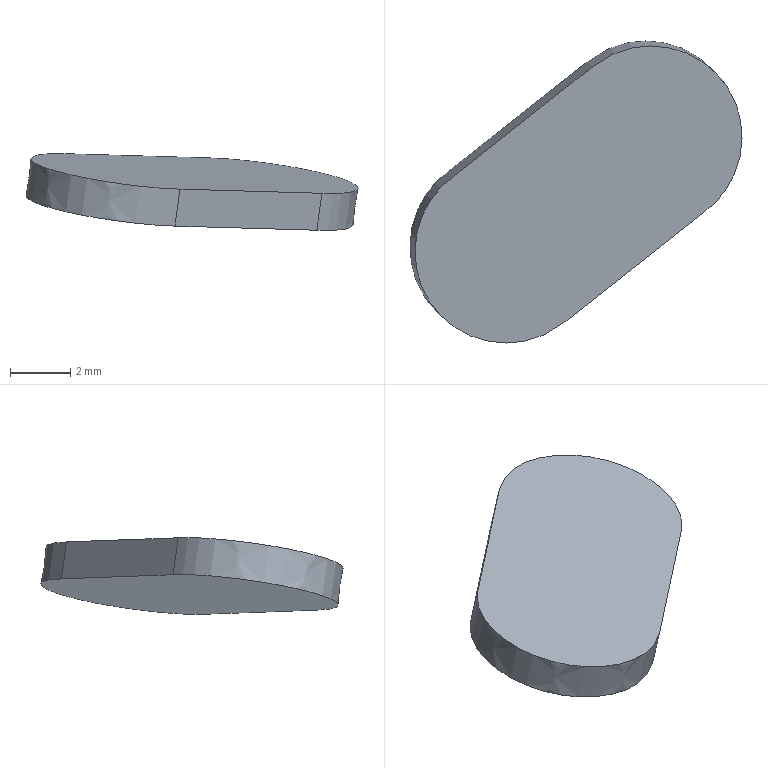Part | STEP file | gslz 2016.10.28-13_id1082_x_t | 1 solid | 6 faces | box 11.029 x 10.034 x 2.548 mm | volume 84.369 mm3 | other 2 | plane 2 | spline 2
STEP:
#1=CARTESIAN_POINT('',(0.,0.,0.));
#2=DIRECTION('',(0.,0.,1.));
#3=DIRECTION('',(1.,0.,0.));
#4=AXIS2_PLACEMENT_3D('',#1,#2,#3);
#5=CARTESIAN_POINT('',(753.441,156.947,-5.848));
#6=VERTEX_POINT('',#5);
#7=CARTESIAN_POINT('',(753.61,156.778,-4.621));
#8=VERTEX_POINT('',#7);
#9=CARTESIAN_POINT('',(753.441,156.947,-5.848));
#10=DIRECTION('',(0.1349,-0.1349,0.9816));
#11=VECTOR('',#10,1.);
#12=LINE('',#9,#11);
#13=CARTESIAN_POINT('',(753.441,156.947,-5.848));
#14=CARTESIAN_POINT('',(753.601,157.072,-5.852));
#15=CARTESIAN_POINT('',(753.942,157.297,-5.868));
#16=CARTESIAN_POINT('',(754.696,157.607,-5.929));
#17=CARTESIAN_POINT('',(755.723,157.678,-6.061));
#18=CARTESIAN_POINT('',(756.89,157.313,-6.271));
#19=CARTESIAN_POINT('',(757.817,156.519,-6.508));
#20=CARTESIAN_POINT('',(758.363,155.425,-6.733));
#21=CARTESIAN_POINT('',(758.438,154.2,-6.912));
#22=CARTESIAN_POINT('',(758.124,153.214,-7.004));
#23=CARTESIAN_POINT('',(757.644,152.553,-7.029));
#24=CARTESIAN_POINT('',(757.346,152.273,-7.027));
#25=CARTESIAN_POINT('',(757.187,152.148,-7.022));
#26=B_SPLINE_CURVE_WITH_KNOTS('',3,(#13,#14,#15,#16,#17,#18,#19,#20,#21,#22,#23,#24,#25),.UNSPECIFIED.,.F.,.F.,(4,1,1,1,1,1,1,1,1,1,4),(0.,0.0625,0.125,0.25,0.375,0.5,0.625,0.75,0.875,0.9375,1.),.UNSPECIFIED.);
#27=DIRECTION('',(0.1349,-0.1349,0.9816));
#28=VECTOR('',#27,1.);
#29=SURFACE_OF_LINEAR_EXTRUSION('',#26,#28);
#30=CARTESIAN_POINT('',(0.,0.));
#31=DIRECTION('',(0.,1.));
#32=VECTOR('',#31,1.);
#33=LINE('',#30,#32);
#34=(GEOMETRIC_REPRESENTATION_CONTEXT(2)PARAMETRIC_REPRESENTATION_CONTEXT()REPRESENTATION_CONTEXT('',''));
#35=DEFINITIONAL_REPRESENTATION('',(#33),#34);
#36=PCURVE('',#29,#35);
#37=CARTESIAN_POINT('',(748.729,153.235,-5.71));
#38=DIRECTION('',(0.6041,-0.7741,-0.1894));
#39=DIRECTION('',(0.7712,0.6278,-0.1058));
#40=AXIS2_PLACEMENT_3D('',#37,#38,#39);
#41=PLANE('',#40);
#42=CARTESIAN_POINT('',(5.979,0.5068));
#43=DIRECTION('',(-0.08446,0.9964));
#44=VECTOR('',#43,1.);
#45=LINE('',#42,#44);
#46=(GEOMETRIC_REPRESENTATION_CONTEXT(2)PARAMETRIC_REPRESENTATION_CONTEXT()REPRESENTATION_CONTEXT('',''));
#47=DEFINITIONAL_REPRESENTATION('',(#45),#46);
#48=PCURVE('',#41,#47);
#49=SURFACE_CURVE('',#12,(#36,#48),.PCURVE_S1.);
#50=EDGE_CURVE('',#6,#8,#49,.T.);
#51=ORIENTED_EDGE('',*,*,#50,.F.);
#52=CARTESIAN_POINT('',(757.187,152.148,-7.022));
#53=VERTEX_POINT('',#52);
#54=CARTESIAN_POINT('',(753.441,156.947,-5.848));
#55=CARTESIAN_POINT('',(753.711,157.16,-5.856));
#56=CARTESIAN_POINT('',(754.017,157.335,-5.873));
#57=CARTESIAN_POINT('',(754.339,157.452,-5.902));
#58=CARTESIAN_POINT('',(754.663,157.568,-5.93));
#59=CARTESIAN_POINT('',(755.012,157.625,-5.97));
#60=CARTESIAN_POINT('',(755.354,157.624,-6.017));
#61=CARTESIAN_POINT('',(755.681,157.623,-6.063));
#62=CARTESIAN_POINT('',(756.012,157.571,-6.115));
#63=CARTESIAN_POINT('',(756.321,157.47,-6.172));
#64=CARTESIAN_POINT('',(756.66,157.361,-6.233));
#65=CARTESIAN_POINT('',(756.982,157.188,-6.301));
#66=CARTESIAN_POINT('',(757.259,156.968,-6.37));
#67=CARTESIAN_POINT('',(757.524,156.757,-6.435));
#68=CARTESIAN_POINT('',(757.756,156.497,-6.503));
#69=CARTESIAN_POINT('',(757.935,156.209,-6.567));
#70=CARTESIAN_POINT('',(758.114,155.92,-6.631));
#71=CARTESIAN_POINT('',(758.247,155.595,-6.694));
#72=CARTESIAN_POINT('',(758.319,155.261,-6.75));
#73=CARTESIAN_POINT('',(758.391,154.929,-6.805));
#74=CARTESIAN_POINT('',(758.406,154.579,-6.855));
#75=CARTESIAN_POINT('',(758.367,154.24,-6.897));
#76=CARTESIAN_POINT('',(758.326,153.889,-6.939));
#77=CARTESIAN_POINT('',(758.227,153.539,-6.974));
#78=CARTESIAN_POINT('',(758.071,153.221,-6.996));
#79=CARTESIAN_POINT('',(757.917,152.909,-7.018));
#80=CARTESIAN_POINT('',(757.703,152.622,-7.028));
#81=CARTESIAN_POINT('',(757.453,152.38,-7.027));
#82=CARTESIAN_POINT('',(757.368,152.298,-7.026));
#83=CARTESIAN_POINT('',(757.279,152.221,-7.025));
#84=CARTESIAN_POINT('',(757.187,152.148,-7.022));
#85=B_SPLINE_CURVE_WITH_KNOTS('',3,(#54,#55,#56,#57,#58,#59,#60,#61,#62,#63,#64,#65,#66,#67,#68,#69,#70,#71,#72,#73,#74,#75,#76,#77,#78,#79,#80,#81,#82,#83,#84),.UNSPECIFIED.,.F.,.F.,(4,3,3,3,3,3,3,3,3,3,4),(0.,0.1062,0.213,0.315,0.4266,0.5332,0.6403,0.7466,0.8564,0.964,1.),.UNSPECIFIED.);
#86=CARTESIAN_POINT('',(0.,0.));
#87=DIRECTION('',(1.,0.));
#88=VECTOR('',#87,1.);
#89=LINE('',#86,#88);
#90=(GEOMETRIC_REPRESENTATION_CONTEXT(2)PARAMETRIC_REPRESENTATION_CONTEXT()REPRESENTATION_CONTEXT('',''));
#91=DEFINITIONAL_REPRESENTATION('',(#89),#90);
#92=PCURVE('',#29,#91);
#93=CARTESIAN_POINT('',(746.154,150.76,-5.696));
#94=CARTESIAN_POINT('',(747.778,149.136,-6.143));
#95=CARTESIAN_POINT('',(749.402,147.512,-6.589));
#96=CARTESIAN_POINT('',(751.026,145.888,-7.036));
#97=CARTESIAN_POINT('',(749.066,153.672,-5.696));
#98=CARTESIAN_POINT('',(750.69,152.048,-6.143));
#99=CARTESIAN_POINT('',(752.314,150.424,-6.589));
#100=CARTESIAN_POINT('',(753.938,148.8,-7.036));
#101=CARTESIAN_POINT('',(751.977,156.583,-5.696));
#102=CARTESIAN_POINT('',(753.601,154.959,-6.143));
#103=CARTESIAN_POINT('',(755.225,153.335,-6.589));
#104=CARTESIAN_POINT('',(756.849,151.711,-7.036));
#105=CARTESIAN_POINT('',(754.889,159.495,-5.696));
#106=CARTESIAN_POINT('',(756.513,157.871,-6.143));
#107=CARTESIAN_POINT('',(758.137,156.247,-6.589));
#108=CARTESIAN_POINT('',(759.761,154.623,-7.036));
#109=B_SPLINE_SURFACE_WITH_KNOTS('',3,3,((#93,#94,#95,#96),(#97,#98,#99,#100),(#101,#102,#103,#104),(#105,#106,#107,#108)),.UNSPECIFIED.,.F.,.F.,.F.,(4,4),(4,4),(0.,1.),(0.,1.),.PIECEWISE_BEZIER_KNOTS.);
#110=CARTESIAN_POINT('',(0.7713,0.1129));
#111=CARTESIAN_POINT('',(0.7772,0.1142));
#112=CARTESIAN_POINT('',(0.789,0.1174));
#113=CARTESIAN_POINT('',(0.8066,0.1243));
#114=CARTESIAN_POINT('',(0.8238,0.1332));
#115=CARTESIAN_POINT('',(0.8407,0.1443));
#116=CARTESIAN_POINT('',(0.8569,0.1575));
#117=CARTESIAN_POINT('',(0.8725,0.1729));
#118=CARTESIAN_POINT('',(0.8875,0.1905));
#119=CARTESIAN_POINT('',(0.9017,0.21));
#120=CARTESIAN_POINT('',(0.915,0.2312));
#121=CARTESIAN_POINT('',(0.9274,0.2539));
#122=CARTESIAN_POINT('',(0.9389,0.2782));
#123=CARTESIAN_POINT('',(0.9494,0.3039));
#124=CARTESIAN_POINT('',(0.959,0.3308));
#125=CARTESIAN_POINT('',(0.9674,0.3586));
#126=CARTESIAN_POINT('',(0.9747,0.3874));
#127=CARTESIAN_POINT('',(0.9808,0.4172));
#128=CARTESIAN_POINT('',(0.9856,0.4476));
#129=CARTESIAN_POINT('',(0.9893,0.4786));
#130=CARTESIAN_POINT('',(0.9916,0.5097));
#131=CARTESIAN_POINT('',(0.9927,0.5412));
#132=CARTESIAN_POINT('',(0.9924,0.5729));
#133=CARTESIAN_POINT('',(0.9909,0.6045));
#134=CARTESIAN_POINT('',(0.9881,0.6357));
#135=CARTESIAN_POINT('',(0.9841,0.6663));
#136=CARTESIAN_POINT('',(0.9788,0.6965));
#137=CARTESIAN_POINT('',(0.9723,0.7261));
#138=CARTESIAN_POINT('',(0.9646,0.7547));
#139=CARTESIAN_POINT('',(0.9558,0.7822));
#140=CARTESIAN_POINT('',(0.9458,0.8083));
#141=CARTESIAN_POINT('',(0.9348,0.8334));
#142=CARTESIAN_POINT('',(0.9228,0.857));
#143=CARTESIAN_POINT('',(0.9099,0.8791));
#144=CARTESIAN_POINT('',(0.8963,0.8995));
#145=CARTESIAN_POINT('',(0.8818,0.9182));
#146=CARTESIAN_POINT('',(0.8667,0.9352));
#147=CARTESIAN_POINT('',(0.8508,0.9502));
#148=CARTESIAN_POINT('',(0.8344,0.9632));
#149=CARTESIAN_POINT('',(0.8177,0.974));
#150=CARTESIAN_POINT('',(0.8004,0.9823));
#151=CARTESIAN_POINT('',(0.7827,0.9884));
#152=CARTESIAN_POINT('',(0.7648,0.9921));
#153=CARTESIAN_POINT('',(0.747,0.9937));
#154=CARTESIAN_POINT('',(0.729,0.993));
#155=CARTESIAN_POINT('',(0.7169,0.9911));
#156=CARTESIAN_POINT('',(0.7109,0.9898));
#157=B_SPLINE_CURVE_WITH_KNOTS('',3,(#110,#111,#112,#113,#114,#115,#116,#117,#118,#119,#120,#121,#122,#123,#124,#125,#126,#127,#128,#129,#130,#131,#132,#133,#134,#135,#136,#137,#138,#139,#140,#141,#142,#143,#144,#145,#146,#147,#148,#149,#150,#151,#152,#153,#154,#155,#156),.UNSPECIFIED.,.F.,.F.,(4,1,1,1,1,1,1,1,1,1,1,1,1,1,1,1,1,1,1,1,1,1,1,1,1,1,1,1,1,1,1,1,1,1,1,1,1,1,1,1,1,1,1,1,4),(0.,0.02273,0.04545,0.06818,0.09091,0.1136,0.1364,0.1591,0.1818,0.2045,0.2273,0.25,0.2727,0.2955,0.3182,0.3409,0.3636,0.3864,0.4091,0.4318,0.4545,0.4773,0.5,0.5227,0.5455,0.5682,0.5909,0.6136,0.6364,0.6591,0.6818,0.7045,0.7273,0.75,0.7727,0.7955,0.8182,0.8409,0.8636,0.8864,0.9091,0.9318,0.9545,0.9773,1.),.QUASI_UNIFORM_KNOTS.);
#158=(GEOMETRIC_REPRESENTATION_CONTEXT(2)PARAMETRIC_REPRESENTATION_CONTEXT()REPRESENTATION_CONTEXT('',''));
#159=DEFINITIONAL_REPRESENTATION('',(#157),#158);
#160=PCURVE('',#109,#159);
#161=SURFACE_CURVE('',#85,(#92,#160),.PCURVE_S1.);
#162=EDGE_CURVE('',#6,#53,#161,.T.);
#163=ORIENTED_EDGE('',*,*,#162,.T.);
#164=CARTESIAN_POINT('',(757.355,151.979,-5.795));
#165=VERTEX_POINT('',#164);
#166=CARTESIAN_POINT('',(757.187,152.148,-7.022));
#167=DIRECTION('',(0.1349,-0.1349,0.9816));
#168=VECTOR('',#167,1.);
#169=LINE('',#166,#168);
#170=CARTESIAN_POINT('',(1.,0.));
#171=DIRECTION('',(0.,1.));
#172=VECTOR('',#171,1.);
#173=LINE('',#170,#172);
#174=(GEOMETRIC_REPRESENTATION_CONTEXT(2)PARAMETRIC_REPRESENTATION_CONTEXT()REPRESENTATION_CONTEXT('',''));
#175=DEFINITIONAL_REPRESENTATION('',(#173),#174);
#176=PCURVE('',#29,#175);
#177=CARTESIAN_POINT('',(757.187,152.148,-7.022));
#178=DIRECTION('',(-0.6041,0.7741,0.1894));
#179=DIRECTION('',(-0.7712,-0.6278,0.1058));
#180=AXIS2_PLACEMENT_3D('',#177,#178,#179);
#181=PLANE('',#180);
#182=CARTESIAN_POINT('',(0.,0.));
#183=DIRECTION('',(0.08446,0.9964));
#184=VECTOR('',#183,1.);
#185=LINE('',#182,#184);
#186=(GEOMETRIC_REPRESENTATION_CONTEXT(2)PARAMETRIC_REPRESENTATION_CONTEXT()REPRESENTATION_CONTEXT('',''));
#187=DEFINITIONAL_REPRESENTATION('',(#185),#186);
#188=PCURVE('',#181,#187);
#189=SURFACE_CURVE('',#169,(#176,#188),.PCURVE_S1.);
#190=EDGE_CURVE('',#53,#165,#189,.T.);
#191=ORIENTED_EDGE('',*,*,#190,.T.);
#192=CARTESIAN_POINT('',(753.61,156.778,-4.621));
#193=CARTESIAN_POINT('',(753.88,156.991,-4.629));
#194=CARTESIAN_POINT('',(754.185,157.167,-4.646));
#195=CARTESIAN_POINT('',(754.508,157.283,-4.675));
#196=CARTESIAN_POINT('',(754.831,157.4,-4.703));
#197=CARTESIAN_POINT('',(755.18,157.457,-4.743));
#198=CARTESIAN_POINT('',(755.522,157.456,-4.79));
#199=CARTESIAN_POINT('',(755.85,157.455,-4.836));
#200=CARTESIAN_POINT('',(756.18,157.402,-4.888));
#201=CARTESIAN_POINT('',(756.49,157.302,-4.945));
#202=CARTESIAN_POINT('',(756.828,157.192,-5.006));
#203=CARTESIAN_POINT('',(757.151,157.02,-5.074));
#204=CARTESIAN_POINT('',(757.428,156.799,-5.143));
#205=CARTESIAN_POINT('',(757.693,156.588,-5.208));
#206=CARTESIAN_POINT('',(757.924,156.328,-5.275));
#207=CARTESIAN_POINT('',(758.103,156.04,-5.34));
#208=CARTESIAN_POINT('',(758.283,155.751,-5.404));
#209=CARTESIAN_POINT('',(758.416,155.426,-5.467));
#210=CARTESIAN_POINT('',(758.488,155.092,-5.523));
#211=CARTESIAN_POINT('',(758.559,154.76,-5.578));
#212=CARTESIAN_POINT('',(758.575,154.41,-5.628));
#213=CARTESIAN_POINT('',(758.535,154.071,-5.67));
#214=CARTESIAN_POINT('',(758.495,153.721,-5.712));
#215=CARTESIAN_POINT('',(758.396,153.37,-5.747));
#216=CARTESIAN_POINT('',(758.239,153.052,-5.769));
#217=CARTESIAN_POINT('',(758.086,152.741,-5.791));
#218=CARTESIAN_POINT('',(757.871,152.454,-5.801));
#219=CARTESIAN_POINT('',(757.622,152.212,-5.8));
#220=CARTESIAN_POINT('',(757.537,152.13,-5.799));
#221=CARTESIAN_POINT('',(757.448,152.052,-5.798));
#222=CARTESIAN_POINT('',(757.355,151.979,-5.795));
#223=B_SPLINE_CURVE_WITH_KNOTS('',3,(#192,#193,#194,#195,#196,#197,#198,#199,#200,#201,#202,#203,#204,#205,#206,#207,#208,#209,#210,#211,#212,#213,#214,#215,#216,#217,#218,#219,#220,#221,#222),.UNSPECIFIED.,.F.,.F.,(4,3,3,3,3,3,3,3,3,3,4),(0.,0.1062,0.213,0.315,0.4266,0.5332,0.6403,0.7466,0.8564,0.964,1.),.UNSPECIFIED.);
#224=CARTESIAN_POINT('',(0.,1.25));
#225=DIRECTION('',(1.,0.));
#226=VECTOR('',#225,1.);
#227=LINE('',#224,#226);
#228=(GEOMETRIC_REPRESENTATION_CONTEXT(2)PARAMETRIC_REPRESENTATION_CONTEXT()REPRESENTATION_CONTEXT('',''));
#229=DEFINITIONAL_REPRESENTATION('',(#227),#228);
#230=PCURVE('',#29,#229);
#231=CARTESIAN_POINT('',(582.842,140.622,16.631));
#232=CARTESIAN_POINT('',(603.987,119.477,10.818));
#233=CARTESIAN_POINT('',(625.133,98.331,5.005));
#234=CARTESIAN_POINT('',(646.279,77.185,-0.8076));
#235=CARTESIAN_POINT('',(667.424,56.039,-6.62));
#236=CARTESIAN_POINT('',(688.57,34.894,-12.433));
#237=CARTESIAN_POINT('',(618.357,176.138,16.631));
#238=CARTESIAN_POINT('',(639.503,154.992,10.818));
#239=CARTESIAN_POINT('',(660.649,133.847,5.005));
#240=CARTESIAN_POINT('',(681.795,112.701,-0.8078));
#241=CARTESIAN_POINT('',(702.94,91.555,-6.621));
#242=CARTESIAN_POINT('',(724.086,70.41,-12.434));
#243=CARTESIAN_POINT('',(653.873,211.654,16.631));
#244=CARTESIAN_POINT('',(675.019,190.508,10.818));
#245=CARTESIAN_POINT('',(696.165,169.363,5.005));
#246=CARTESIAN_POINT('',(717.31,148.217,-0.808));
#247=CARTESIAN_POINT('',(738.456,127.071,-6.621));
#248=CARTESIAN_POINT('',(759.602,105.925,-12.434));
#249=CARTESIAN_POINT('',(689.389,247.17,16.63));
#250=CARTESIAN_POINT('',(710.535,226.024,10.818));
#251=CARTESIAN_POINT('',(731.68,204.878,5.005));
#252=CARTESIAN_POINT('',(752.826,183.733,-0.8082));
#253=CARTESIAN_POINT('',(773.972,162.587,-6.621));
#254=CARTESIAN_POINT('',(795.118,141.441,-12.434));
#255=CARTESIAN_POINT('',(724.905,282.686,16.63));
#256=CARTESIAN_POINT('',(746.051,261.54,10.817));
#257=CARTESIAN_POINT('',(767.196,240.394,5.005));
#258=CARTESIAN_POINT('',(788.342,219.248,-0.8083));
#259=CARTESIAN_POINT('',(809.488,198.103,-6.621));
#260=CARTESIAN_POINT('',(830.633,176.957,-12.434));
#261=CARTESIAN_POINT('',(760.421,318.201,16.63));
#262=CARTESIAN_POINT('',(781.566,297.056,10.817));
#263=CARTESIAN_POINT('',(802.712,275.91,5.004));
#264=CARTESIAN_POINT('',(823.858,254.764,-0.8085));
#265=CARTESIAN_POINT('',(845.003,233.618,-6.621));
#266=CARTESIAN_POINT('',(866.149,212.473,-12.434));
#267=B_SPLINE_SURFACE_WITH_KNOTS('',5,5,((#231,#232,#233,#234,#235,#236),(#237,#238,#239,#240,#241,#242),(#243,#244,#245,#246,#247,#248),(#249,#250,#251,#252,#253,#254),(#255,#256,#257,#258,#259,#260),(#261,#262,#263,#264,#265,#266)),.UNSPECIFIED.,.F.,.F.,.F.,(6,6),(6,6),(0.,1.),(0.,1.),.PIECEWISE_BEZIER_KNOTS.);
#268=CARTESIAN_POINT('',(0.5263,0.7312));
#269=CARTESIAN_POINT('',(0.5266,0.7312));
#270=CARTESIAN_POINT('',(0.5272,0.7314));
#271=CARTESIAN_POINT('',(0.528,0.7317));
#272=CARTESIAN_POINT('',(0.5289,0.7321));
#273=CARTESIAN_POINT('',(0.5297,0.7326));
#274=CARTESIAN_POINT('',(0.5305,0.7332));
#275=CARTESIAN_POINT('',(0.5313,0.7339));
#276=CARTESIAN_POINT('',(0.532,0.7348));
#277=CARTESIAN_POINT('',(0.5327,0.7356));
#278=CARTESIAN_POINT('',(0.5334,0.7366));
#279=CARTESIAN_POINT('',(0.534,0.7377));
#280=CARTESIAN_POINT('',(0.5346,0.7388));
#281=CARTESIAN_POINT('',(0.5351,0.74));
#282=CARTESIAN_POINT('',(0.5355,0.7412));
#283=CARTESIAN_POINT('',(0.536,0.7425));
#284=CARTESIAN_POINT('',(0.5363,0.7438));
#285=CARTESIAN_POINT('',(0.5366,0.7452));
#286=CARTESIAN_POINT('',(0.5369,0.7466));
#287=CARTESIAN_POINT('',(0.537,0.748));
#288=CARTESIAN_POINT('',(0.5372,0.7495));
#289=CARTESIAN_POINT('',(0.5372,0.7509));
#290=CARTESIAN_POINT('',(0.5372,0.7524));
#291=CARTESIAN_POINT('',(0.5371,0.7538));
#292=CARTESIAN_POINT('',(0.537,0.7553));
#293=CARTESIAN_POINT('',(0.5368,0.7567));
#294=CARTESIAN_POINT('',(0.5365,0.7581));
#295=CARTESIAN_POINT('',(0.5362,0.7594));
#296=CARTESIAN_POINT('',(0.5358,0.7607));
#297=CARTESIAN_POINT('',(0.5354,0.762));
#298=CARTESIAN_POINT('',(0.5349,0.7632));
#299=CARTESIAN_POINT('',(0.5344,0.7644));
#300=CARTESIAN_POINT('',(0.5338,0.7655));
#301=CARTESIAN_POINT('',(0.5331,0.7665));
#302=CARTESIAN_POINT('',(0.5325,0.7674));
#303=CARTESIAN_POINT('',(0.5318,0.7683));
#304=CARTESIAN_POINT('',(0.531,0.7691));
#305=CARTESIAN_POINT('',(0.5302,0.7698));
#306=CARTESIAN_POINT('',(0.5294,0.7704));
#307=CARTESIAN_POINT('',(0.5286,0.7709));
#308=CARTESIAN_POINT('',(0.5277,0.7712));
#309=CARTESIAN_POINT('',(0.5269,0.7715));
#310=CARTESIAN_POINT('',(0.526,0.7717));
#311=CARTESIAN_POINT('',(0.5251,0.7718));
#312=CARTESIAN_POINT('',(0.5242,0.7717));
#313=CARTESIAN_POINT('',(0.5236,0.7716));
#314=CARTESIAN_POINT('',(0.5233,0.7716));
#315=B_SPLINE_CURVE_WITH_KNOTS('',3,(#268,#269,#270,#271,#272,#273,#274,#275,#276,#277,#278,#279,#280,#281,#282,#283,#284,#285,#286,#287,#288,#289,#290,#291,#292,#293,#294,#295,#296,#297,#298,#299,#300,#301,#302,#303,#304,#305,#306,#307,#308,#309,#310,#311,#312,#313,#314),.UNSPECIFIED.,.F.,.F.,(4,1,1,1,1,1,1,1,1,1,1,1,1,1,1,1,1,1,1,1,1,1,1,1,1,1,1,1,1,1,1,1,1,1,1,1,1,1,1,1,1,1,1,1,4),(0.,0.02273,0.04545,0.06818,0.09091,0.1136,0.1364,0.1591,0.1818,0.2045,0.2273,0.25,0.2727,0.2955,0.3182,0.3409,0.3636,0.3864,0.4091,0.4318,0.4545,0.4773,0.5,0.5227,0.5455,0.5682,0.5909,0.6136,0.6364,0.6591,0.6818,0.7045,0.7273,0.75,0.7727,0.7955,0.8182,0.8409,0.8636,0.8864,0.9091,0.9318,0.9545,0.9773,1.),.QUASI_UNIFORM_KNOTS.);
#316=(GEOMETRIC_REPRESENTATION_CONTEXT(2)PARAMETRIC_REPRESENTATION_CONTEXT()REPRESENTATION_CONTEXT('',''));
#317=DEFINITIONAL_REPRESENTATION('',(#315),#316);
#318=PCURVE('',#267,#317);
#319=SURFACE_CURVE('',#223,(#230,#318),.PCURVE_S1.);
#320=EDGE_CURVE('',#8,#165,#319,.T.);
#321=ORIENTED_EDGE('',*,*,#320,.F.);
#322=EDGE_LOOP('',(#51,#163,#191,#321));
#323=FACE_BOUND('',#322,.F.);
#324=ADVANCED_FACE('',(#323),#29,.F.);
#325=CARTESIAN_POINT('',(752.643,148.268,-5.657));
#326=VERTEX_POINT('',#325);
#327=CARTESIAN_POINT('',(757.355,151.979,-5.795));
#328=CARTESIAN_POINT('',(755.784,150.742,-5.749));
#329=CARTESIAN_POINT('',(754.214,149.505,-5.703));
#330=CARTESIAN_POINT('',(752.643,148.268,-5.657));
#331=B_SPLINE_CURVE_WITH_KNOTS('',3,(#327,#328,#329,#330),.UNSPECIFIED.,.F.,.F.,(4,4),(0.,1.),.PIECEWISE_BEZIER_KNOTS.);
#332=CARTESIAN_POINT('',(0.1056,1.246));
#333=CARTESIAN_POINT('',(2.098,1.077));
#334=CARTESIAN_POINT('',(4.091,0.9077));
#335=CARTESIAN_POINT('',(6.084,0.7388));
#336=B_SPLINE_CURVE_WITH_KNOTS('',3,(#332,#333,#334,#335),.UNSPECIFIED.,.F.,.F.,(4,4),(0.,1.),.PIECEWISE_BEZIER_KNOTS.);
#337=(GEOMETRIC_REPRESENTATION_CONTEXT(2)PARAMETRIC_REPRESENTATION_CONTEXT()REPRESENTATION_CONTEXT('',''));
#338=DEFINITIONAL_REPRESENTATION('',(#336),#337);
#339=PCURVE('',#181,#338);
#340=CARTESIAN_POINT('',(0.5233,0.7716));
#341=CARTESIAN_POINT('',(0.4996,0.7668));
#342=B_SPLINE_CURVE_WITH_KNOTS('',1,(#340,#341),.UNSPECIFIED.,.F.,.F.,(2,2),(0.,1.),.PIECEWISE_BEZIER_KNOTS.);
#343=(GEOMETRIC_REPRESENTATION_CONTEXT(2)PARAMETRIC_REPRESENTATION_CONTEXT()REPRESENTATION_CONTEXT('',''));
#344=DEFINITIONAL_REPRESENTATION('',(#342),#343);
#345=PCURVE('',#267,#344);
#346=SURFACE_CURVE('',#331,(#339,#345),.PCURVE_S1.);
#347=EDGE_CURVE('',#165,#326,#346,.T.);
#348=ORIENTED_EDGE('',*,*,#347,.T.);
#349=CARTESIAN_POINT('',(752.474,148.436,-6.884));
#350=VERTEX_POINT('',#349);
#351=CARTESIAN_POINT('',(752.474,148.436,-6.884));
#352=DIRECTION('',(0.1349,-0.1349,0.9816));
#353=VECTOR('',#352,1.);
#354=LINE('',#351,#353);
#355=CARTESIAN_POINT('',(5.979,-0.5068));
#356=DIRECTION('',(0.08446,0.9964));
#357=VECTOR('',#356,1.);
#358=LINE('',#355,#357);
#359=(GEOMETRIC_REPRESENTATION_CONTEXT(2)PARAMETRIC_REPRESENTATION_CONTEXT()REPRESENTATION_CONTEXT('',''));
#360=DEFINITIONAL_REPRESENTATION('',(#358),#359);
#361=PCURVE('',#181,#360);
#362=CARTESIAN_POINT('',(752.474,148.436,-6.884));
#363=CARTESIAN_POINT('',(752.315,148.311,-6.88));
#364=CARTESIAN_POINT('',(751.973,148.086,-6.864));
#365=CARTESIAN_POINT('',(751.22,147.776,-6.803));
#366=CARTESIAN_POINT('',(750.192,147.705,-6.671));
#367=CARTESIAN_POINT('',(749.026,148.07,-6.461));
#368=CARTESIAN_POINT('',(748.098,148.865,-6.224));
#369=CARTESIAN_POINT('',(747.552,149.959,-5.999));
#370=CARTESIAN_POINT('',(747.477,151.183,-5.82));
#371=CARTESIAN_POINT('',(747.792,152.169,-5.728));
#372=CARTESIAN_POINT('',(748.271,152.831,-5.703));
#373=CARTESIAN_POINT('',(748.569,153.11,-5.705));
#374=CARTESIAN_POINT('',(748.729,153.235,-5.71));
#375=B_SPLINE_CURVE_WITH_KNOTS('',3,(#362,#363,#364,#365,#366,#367,#368,#369,#370,#371,#372,#373,#374),.UNSPECIFIED.,.F.,.F.,(4,1,1,1,1,1,1,1,1,1,4),(0.,0.0625,0.125,0.25,0.375,0.5,0.625,0.75,0.875,0.9375,1.),.UNSPECIFIED.);
#376=DIRECTION('',(0.1349,-0.1349,0.9816));
#377=VECTOR('',#376,1.);
#378=SURFACE_OF_LINEAR_EXTRUSION('',#375,#377);
#379=CARTESIAN_POINT('',(0.,0.));
#380=DIRECTION('',(0.,1.));
#381=VECTOR('',#380,1.);
#382=LINE('',#379,#381);
#383=(GEOMETRIC_REPRESENTATION_CONTEXT(2)PARAMETRIC_REPRESENTATION_CONTEXT()REPRESENTATION_CONTEXT('',''));
#384=DEFINITIONAL_REPRESENTATION('',(#382),#383);
#385=PCURVE('',#378,#384);
#386=SURFACE_CURVE('',#354,(#361,#385),.PCURVE_S1.);
#387=EDGE_CURVE('',#350,#326,#386,.T.);
#388=ORIENTED_EDGE('',*,*,#387,.F.);
#389=CARTESIAN_POINT('',(757.187,152.148,-7.022));
#390=CARTESIAN_POINT('',(755.616,150.911,-6.976));
#391=CARTESIAN_POINT('',(754.045,149.673,-6.93));
#392=CARTESIAN_POINT('',(752.474,148.436,-6.884));
#393=B_SPLINE_CURVE_WITH_KNOTS('',3,(#389,#390,#391,#392),.UNSPECIFIED.,.F.,.F.,(4,4),(0.,1.),.PIECEWISE_BEZIER_KNOTS.);
#394=CARTESIAN_POINT('',(0.,0.));
#395=CARTESIAN_POINT('',(1.993,-0.1689));
#396=CARTESIAN_POINT('',(3.986,-0.3379));
#397=CARTESIAN_POINT('',(5.979,-0.5068));
#398=B_SPLINE_CURVE_WITH_KNOTS('',3,(#394,#395,#396,#397),.UNSPECIFIED.,.F.,.F.,(4,4),(0.,1.),.PIECEWISE_BEZIER_KNOTS.);
#399=(GEOMETRIC_REPRESENTATION_CONTEXT(2)PARAMETRIC_REPRESENTATION_CONTEXT()REPRESENTATION_CONTEXT('',''));
#400=DEFINITIONAL_REPRESENTATION('',(#398),#399);
#401=PCURVE('',#181,#400);
#402=CARTESIAN_POINT('',(0.7109,0.9898));
#403=CARTESIAN_POINT('',(0.2287,0.8871));
#404=B_SPLINE_CURVE_WITH_KNOTS('',1,(#402,#403),.UNSPECIFIED.,.F.,.F.,(2,2),(0.,1.),.PIECEWISE_BEZIER_KNOTS.);
#405=(GEOMETRIC_REPRESENTATION_CONTEXT(2)PARAMETRIC_REPRESENTATION_CONTEXT()REPRESENTATION_CONTEXT('',''));
#406=DEFINITIONAL_REPRESENTATION('',(#404),#405);
#407=PCURVE('',#109,#406);
#408=SURFACE_CURVE('',#393,(#401,#407),.PCURVE_S1.);
#409=EDGE_CURVE('',#53,#350,#408,.T.);
#410=ORIENTED_EDGE('',*,*,#409,.F.);
#411=ORIENTED_EDGE('',*,*,#190,.T.);
#412=EDGE_LOOP('',(#348,#388,#410,#411));
#413=FACE_BOUND('',#412,.T.);
#414=ADVANCED_FACE('',(#413),#181,.F.);
#415=ORIENTED_EDGE('',*,*,#387,.F.);
#416=CARTESIAN_POINT('',(748.729,153.235,-5.71));
#417=VERTEX_POINT('',#416);
#418=CARTESIAN_POINT('',(752.474,148.436,-6.884));
#419=CARTESIAN_POINT('',(752.204,148.224,-6.877));
#420=CARTESIAN_POINT('',(751.898,148.048,-6.859));
#421=CARTESIAN_POINT('',(751.576,147.932,-6.83));
#422=CARTESIAN_POINT('',(751.252,147.815,-6.802));
#423=CARTESIAN_POINT('',(750.903,147.758,-6.762));
#424=CARTESIAN_POINT('',(750.562,147.759,-6.715));
#425=CARTESIAN_POINT('',(750.234,147.76,-6.67));
#426=CARTESIAN_POINT('',(749.904,147.812,-6.617));
#427=CARTESIAN_POINT('',(749.594,147.913,-6.56));
#428=CARTESIAN_POINT('',(749.256,148.023,-6.499));
#429=CARTESIAN_POINT('',(748.933,148.195,-6.431));
#430=CARTESIAN_POINT('',(748.656,148.416,-6.363));
#431=CARTESIAN_POINT('',(748.391,148.627,-6.297));
#432=CARTESIAN_POINT('',(748.16,148.886,-6.23));
#433=CARTESIAN_POINT('',(747.981,149.174,-6.165));
#434=CARTESIAN_POINT('',(747.801,149.463,-6.101));
#435=CARTESIAN_POINT('',(747.668,149.788,-6.038));
#436=CARTESIAN_POINT('',(747.596,150.123,-5.982));
#437=CARTESIAN_POINT('',(747.525,150.455,-5.927));
#438=CARTESIAN_POINT('',(747.509,150.804,-5.877));
#439=CARTESIAN_POINT('',(747.548,151.144,-5.835));
#440=CARTESIAN_POINT('',(747.589,151.494,-5.793));
#441=CARTESIAN_POINT('',(747.688,151.844,-5.758));
#442=CARTESIAN_POINT('',(747.845,152.163,-5.736));
#443=CARTESIAN_POINT('',(747.998,152.474,-5.714));
#444=CARTESIAN_POINT('',(748.212,152.761,-5.704));
#445=CARTESIAN_POINT('',(748.462,153.003,-5.705));
#446=CARTESIAN_POINT('',(748.547,153.085,-5.706));
#447=CARTESIAN_POINT('',(748.636,153.163,-5.707));
#448=CARTESIAN_POINT('',(748.729,153.235,-5.71));
#449=B_SPLINE_CURVE_WITH_KNOTS('',3,(#418,#419,#420,#421,#422,#423,#424,#425,#426,#427,#428,#429,#430,#431,#432,#433,#434,#435,#436,#437,#438,#439,#440,#441,#442,#443,#444,#445,#446,#447,#448),.UNSPECIFIED.,.F.,.F.,(4,3,3,3,3,3,3,3,3,3,4),(0.,0.1062,0.213,0.315,0.4266,0.5332,0.6403,0.7466,0.8564,0.964,1.),.UNSPECIFIED.);
#450=CARTESIAN_POINT('',(0.,0.));
#451=DIRECTION('',(1.,0.));
#452=VECTOR('',#451,1.);
#453=LINE('',#450,#452);
#454=(GEOMETRIC_REPRESENTATION_CONTEXT(2)PARAMETRIC_REPRESENTATION_CONTEXT()REPRESENTATION_CONTEXT('',''));
#455=DEFINITIONAL_REPRESENTATION('',(#453),#454);
#456=PCURVE('',#378,#455);
#457=CARTESIAN_POINT('',(0.2287,0.8871));
#458=CARTESIAN_POINT('',(0.2228,0.8858));
#459=CARTESIAN_POINT('',(0.211,0.8826));
#460=CARTESIAN_POINT('',(0.1934,0.8757));
#461=CARTESIAN_POINT('',(0.1762,0.8668));
#462=CARTESIAN_POINT('',(0.1593,0.8557));
#463=CARTESIAN_POINT('',(0.1431,0.8425));
#464=CARTESIAN_POINT('',(0.1275,0.8271));
#465=CARTESIAN_POINT('',(0.1125,0.8095));
#466=CARTESIAN_POINT('',(0.09832,0.79));
#467=CARTESIAN_POINT('',(0.08501,0.7688));
#468=CARTESIAN_POINT('',(0.07264,0.7461));
#469=CARTESIAN_POINT('',(0.06112,0.7218));
#470=CARTESIAN_POINT('',(0.05055,0.6961));
#471=CARTESIAN_POINT('',(0.04102,0.6692));
#472=CARTESIAN_POINT('',(0.03259,0.6414));
#473=CARTESIAN_POINT('',(0.02535,0.6126));
#474=CARTESIAN_POINT('',(0.01924,0.5828));
#475=CARTESIAN_POINT('',(0.01435,0.5524));
#476=CARTESIAN_POINT('',(0.01071,0.5214));
#477=CARTESIAN_POINT('',(0.008384,0.4903));
#478=CARTESIAN_POINT('',(0.007344,0.4588));
#479=CARTESIAN_POINT('',(0.00758,0.4271));
#480=CARTESIAN_POINT('',(0.009087,0.3955));
#481=CARTESIAN_POINT('',(0.01186,0.3643));
#482=CARTESIAN_POINT('',(0.01589,0.3337));
#483=CARTESIAN_POINT('',(0.0212,0.3035));
#484=CARTESIAN_POINT('',(0.02772,0.2739));
#485=CARTESIAN_POINT('',(0.03541,0.2453));
#486=CARTESIAN_POINT('',(0.04423,0.2178));
#487=CARTESIAN_POINT('',(0.05416,0.1917));
#488=CARTESIAN_POINT('',(0.06519,0.1666));
#489=CARTESIAN_POINT('',(0.0772,0.143));
#490=CARTESIAN_POINT('',(0.09009,0.1209));
#491=CARTESIAN_POINT('',(0.1037,0.1005));
#492=CARTESIAN_POINT('',(0.1182,0.08181));
#493=CARTESIAN_POINT('',(0.1333,0.06483));
#494=CARTESIAN_POINT('',(0.1492,0.04976));
#495=CARTESIAN_POINT('',(0.1656,0.03676));
#496=CARTESIAN_POINT('',(0.1823,0.02602));
#497=CARTESIAN_POINT('',(0.1996,0.01766));
#498=CARTESIAN_POINT('',(0.2173,0.01161));
#499=CARTESIAN_POINT('',(0.2352,0.007852));
#500=CARTESIAN_POINT('',(0.253,0.006334));
#501=CARTESIAN_POINT('',(0.271,0.007038));
#502=CARTESIAN_POINT('',(0.2831,0.00891));
#503=CARTESIAN_POINT('',(0.2891,0.01018));
#504=B_SPLINE_CURVE_WITH_KNOTS('',3,(#457,#458,#459,#460,#461,#462,#463,#464,#465,#466,#467,#468,#469,#470,#471,#472,#473,#474,#475,#476,#477,#478,#479,#480,#481,#482,#483,#484,#485,#486,#487,#488,#489,#490,#491,#492,#493,#494,#495,#496,#497,#498,#499,#500,#501,#502,#503),.UNSPECIFIED.,.F.,.F.,(4,1,1,1,1,1,1,1,1,1,1,1,1,1,1,1,1,1,1,1,1,1,1,1,1,1,1,1,1,1,1,1,1,1,1,1,1,1,1,1,1,1,1,1,4),(0.,0.02273,0.04545,0.06818,0.09091,0.1136,0.1364,0.1591,0.1818,0.2045,0.2273,0.25,0.2727,0.2955,0.3182,0.3409,0.3636,0.3864,0.4091,0.4318,0.4545,0.4773,0.5,0.5227,0.5455,0.5682,0.5909,0.6136,0.6364,0.6591,0.6818,0.7045,0.7273,0.75,0.7727,0.7955,0.8182,0.8409,0.8636,0.8864,0.9091,0.9318,0.9545,0.9773,1.),.QUASI_UNIFORM_KNOTS.);
#505=(GEOMETRIC_REPRESENTATION_CONTEXT(2)PARAMETRIC_REPRESENTATION_CONTEXT()REPRESENTATION_CONTEXT('',''));
#506=DEFINITIONAL_REPRESENTATION('',(#504),#505);
#507=PCURVE('',#109,#506);
#508=SURFACE_CURVE('',#449,(#456,#507),.PCURVE_S1.);
#509=EDGE_CURVE('',#350,#417,#508,.T.);
#510=ORIENTED_EDGE('',*,*,#509,.T.);
#511=CARTESIAN_POINT('',(748.897,153.067,-4.483));
#512=VERTEX_POINT('',#511);
#513=CARTESIAN_POINT('',(748.729,153.235,-5.71));
#514=DIRECTION('',(0.1349,-0.1349,0.9816));
#515=VECTOR('',#514,1.);
#516=LINE('',#513,#515);
#517=CARTESIAN_POINT('',(1.,0.));
#518=DIRECTION('',(0.,1.));
#519=VECTOR('',#518,1.);
#520=LINE('',#517,#519);
#521=(GEOMETRIC_REPRESENTATION_CONTEXT(2)PARAMETRIC_REPRESENTATION_CONTEXT()REPRESENTATION_CONTEXT('',''));
#522=DEFINITIONAL_REPRESENTATION('',(#520),#521);
#523=PCURVE('',#378,#522);
#524=CARTESIAN_POINT('',(0.,0.));
#525=DIRECTION('',(-0.08446,0.9964));
#526=VECTOR('',#525,1.);
#527=LINE('',#524,#526);
#528=(GEOMETRIC_REPRESENTATION_CONTEXT(2)PARAMETRIC_REPRESENTATION_CONTEXT()REPRESENTATION_CONTEXT('',''));
#529=DEFINITIONAL_REPRESENTATION('',(#527),#528);
#530=PCURVE('',#41,#529);
#531=SURFACE_CURVE('',#516,(#523,#530),.PCURVE_S1.);
#532=EDGE_CURVE('',#417,#512,#531,.T.);
#533=ORIENTED_EDGE('',*,*,#532,.T.);
#534=CARTESIAN_POINT('',(752.643,148.268,-5.657));
#535=CARTESIAN_POINT('',(752.373,148.055,-5.65));
#536=CARTESIAN_POINT('',(752.067,147.879,-5.632));
#537=CARTESIAN_POINT('',(751.745,147.763,-5.603));
#538=CARTESIAN_POINT('',(751.421,147.646,-5.575));
#539=CARTESIAN_POINT('',(751.072,147.589,-5.535));
#540=CARTESIAN_POINT('',(750.73,147.59,-5.488));
#541=CARTESIAN_POINT('',(750.403,147.591,-5.443));
#542=CARTESIAN_POINT('',(750.072,147.644,-5.39));
#543=CARTESIAN_POINT('',(749.762,147.744,-5.333));
#544=CARTESIAN_POINT('',(749.424,147.854,-5.272));
#545=CARTESIAN_POINT('',(749.102,148.026,-5.204));
#546=CARTESIAN_POINT('',(748.825,148.247,-5.135));
#547=CARTESIAN_POINT('',(748.56,148.458,-5.07));
#548=CARTESIAN_POINT('',(748.328,148.718,-5.003));
#549=CARTESIAN_POINT('',(748.149,149.005,-4.938));
#550=CARTESIAN_POINT('',(747.969,149.295,-4.874));
#551=CARTESIAN_POINT('',(747.837,149.62,-4.811));
#552=CARTESIAN_POINT('',(747.765,149.954,-4.755));
#553=CARTESIAN_POINT('',(747.693,150.286,-4.7));
#554=CARTESIAN_POINT('',(747.678,150.635,-4.65));
#555=CARTESIAN_POINT('',(747.717,150.975,-4.608));
#556=CARTESIAN_POINT('',(747.757,151.325,-4.566));
#557=CARTESIAN_POINT('',(747.857,151.676,-4.531));
#558=CARTESIAN_POINT('',(748.013,151.994,-4.509));
#559=CARTESIAN_POINT('',(748.166,152.305,-4.487));
#560=CARTESIAN_POINT('',(748.381,152.592,-4.477));
#561=CARTESIAN_POINT('',(748.631,152.834,-4.478));
#562=CARTESIAN_POINT('',(748.716,152.916,-4.479));
#563=CARTESIAN_POINT('',(748.805,152.994,-4.48));
#564=CARTESIAN_POINT('',(748.897,153.067,-4.483));
#565=B_SPLINE_CURVE_WITH_KNOTS('',3,(#534,#535,#536,#537,#538,#539,#540,#541,#542,#543,#544,#545,#546,#547,#548,#549,#550,#551,#552,#553,#554,#555,#556,#557,#558,#559,#560,#561,#562,#563,#564),.UNSPECIFIED.,.F.,.F.,(4,3,3,3,3,3,3,3,3,3,4),(0.,0.1062,0.213,0.315,0.4266,0.5332,0.6403,0.7466,0.8564,0.964,1.),.UNSPECIFIED.);
#566=CARTESIAN_POINT('',(0.,1.25));
#567=DIRECTION('',(1.,0.));
#568=VECTOR('',#567,1.);
#569=LINE('',#566,#568);
#570=(GEOMETRIC_REPRESENTATION_CONTEXT(2)PARAMETRIC_REPRESENTATION_CONTEXT()REPRESENTATION_CONTEXT('',''));
#571=DEFINITIONAL_REPRESENTATION('',(#569),#570);
#572=PCURVE('',#378,#571);
#573=CARTESIAN_POINT('',(0.4996,0.7668));
#574=CARTESIAN_POINT('',(0.4993,0.7668));
#575=CARTESIAN_POINT('',(0.4988,0.7666));
#576=CARTESIAN_POINT('',(0.4979,0.7663));
#577=CARTESIAN_POINT('',(0.497,0.7659));
#578=CARTESIAN_POINT('',(0.4962,0.7654));
#579=CARTESIAN_POINT('',(0.4954,0.7648));
#580=CARTESIAN_POINT('',(0.4946,0.7641));
#581=CARTESIAN_POINT('',(0.4939,0.7633));
#582=CARTESIAN_POINT('',(0.4932,0.7624));
#583=CARTESIAN_POINT('',(0.4926,0.7614));
#584=CARTESIAN_POINT('',(0.4919,0.7604));
#585=CARTESIAN_POINT('',(0.4914,0.7592));
#586=CARTESIAN_POINT('',(0.4909,0.758));
#587=CARTESIAN_POINT('',(0.4904,0.7568));
#588=CARTESIAN_POINT('',(0.49,0.7555));
#589=CARTESIAN_POINT('',(0.4896,0.7542));
#590=CARTESIAN_POINT('',(0.4893,0.7528));
#591=CARTESIAN_POINT('',(0.4891,0.7514));
#592=CARTESIAN_POINT('',(0.4889,0.75));
#593=CARTESIAN_POINT('',(0.4888,0.7486));
#594=CARTESIAN_POINT('',(0.4887,0.7471));
#595=CARTESIAN_POINT('',(0.4887,0.7457));
#596=CARTESIAN_POINT('',(0.4888,0.7442));
#597=CARTESIAN_POINT('',(0.489,0.7428));
#598=CARTESIAN_POINT('',(0.4892,0.7413));
#599=CARTESIAN_POINT('',(0.4894,0.74));
#600=CARTESIAN_POINT('',(0.4897,0.7386));
#601=CARTESIAN_POINT('',(0.4901,0.7373));
#602=CARTESIAN_POINT('',(0.4906,0.736));
#603=CARTESIAN_POINT('',(0.491,0.7348));
#604=CARTESIAN_POINT('',(0.4916,0.7337));
#605=CARTESIAN_POINT('',(0.4922,0.7326));
#606=CARTESIAN_POINT('',(0.4928,0.7315));
#607=CARTESIAN_POINT('',(0.4935,0.7306));
#608=CARTESIAN_POINT('',(0.4942,0.7297));
#609=CARTESIAN_POINT('',(0.4949,0.729));
#610=CARTESIAN_POINT('',(0.4957,0.7283));
#611=CARTESIAN_POINT('',(0.4965,0.7277));
#612=CARTESIAN_POINT('',(0.4973,0.7272));
#613=CARTESIAN_POINT('',(0.4982,0.7268));
#614=CARTESIAN_POINT('',(0.4991,0.7265));
#615=CARTESIAN_POINT('',(0.4999,0.7263));
#616=CARTESIAN_POINT('',(0.5008,0.7263));
#617=CARTESIAN_POINT('',(0.5017,0.7263));
#618=CARTESIAN_POINT('',(0.5023,0.7264));
#619=CARTESIAN_POINT('',(0.5026,0.7264));
#620=B_SPLINE_CURVE_WITH_KNOTS('',3,(#573,#574,#575,#576,#577,#578,#579,#580,#581,#582,#583,#584,#585,#586,#587,#588,#589,#590,#591,#592,#593,#594,#595,#596,#597,#598,#599,#600,#601,#602,#603,#604,#605,#606,#607,#608,#609,#610,#611,#612,#613,#614,#615,#616,#617,#618,#619),.UNSPECIFIED.,.F.,.F.,(4,1,1,1,1,1,1,1,1,1,1,1,1,1,1,1,1,1,1,1,1,1,1,1,1,1,1,1,1,1,1,1,1,1,1,1,1,1,1,1,1,1,1,1,4),(0.,0.02273,0.04545,0.06818,0.09091,0.1136,0.1364,0.1591,0.1818,0.2045,0.2273,0.25,0.2727,0.2955,0.3182,0.3409,0.3636,0.3864,0.4091,0.4318,0.4545,0.4773,0.5,0.5227,0.5455,0.5682,0.5909,0.6136,0.6364,0.6591,0.6818,0.7045,0.7273,0.75,0.7727,0.7955,0.8182,0.8409,0.8636,0.8864,0.9091,0.9318,0.9545,0.9773,1.),.QUASI_UNIFORM_KNOTS.);
#621=(GEOMETRIC_REPRESENTATION_CONTEXT(2)PARAMETRIC_REPRESENTATION_CONTEXT()REPRESENTATION_CONTEXT('',''));
#622=DEFINITIONAL_REPRESENTATION('',(#620),#621);
#623=PCURVE('',#267,#622);
#624=SURFACE_CURVE('',#565,(#572,#623),.PCURVE_S1.);
#625=EDGE_CURVE('',#326,#512,#624,.T.);
#626=ORIENTED_EDGE('',*,*,#625,.F.);
#627=EDGE_LOOP('',(#415,#510,#533,#626));
#628=FACE_BOUND('',#627,.F.);
#629=ADVANCED_FACE('',(#628),#378,.F.);
#630=CARTESIAN_POINT('',(748.897,153.067,-4.483));
#631=CARTESIAN_POINT('',(750.468,154.304,-4.529));
#632=CARTESIAN_POINT('',(752.039,155.541,-4.575));
#633=CARTESIAN_POINT('',(753.61,156.778,-4.621));
#634=B_SPLINE_CURVE_WITH_KNOTS('',3,(#630,#631,#632,#633),.UNSPECIFIED.,.F.,.F.,(4,4),(0.,1.),.PIECEWISE_BEZIER_KNOTS.);
#635=CARTESIAN_POINT('',(-0.1056,1.246));
#636=CARTESIAN_POINT('',(1.887,1.414));
#637=CARTESIAN_POINT('',(3.88,1.583));
#638=CARTESIAN_POINT('',(5.873,1.752));
#639=B_SPLINE_CURVE_WITH_KNOTS('',3,(#635,#636,#637,#638),.UNSPECIFIED.,.F.,.F.,(4,4),(0.,1.),.PIECEWISE_BEZIER_KNOTS.);
#640=(GEOMETRIC_REPRESENTATION_CONTEXT(2)PARAMETRIC_REPRESENTATION_CONTEXT()REPRESENTATION_CONTEXT('',''));
#641=DEFINITIONAL_REPRESENTATION('',(#639),#640);
#642=PCURVE('',#41,#641);
#643=CARTESIAN_POINT('',(0.5026,0.7264));
#644=CARTESIAN_POINT('',(0.5263,0.7312));
#645=B_SPLINE_CURVE_WITH_KNOTS('',1,(#643,#644),.UNSPECIFIED.,.F.,.F.,(2,2),(0.,1.),.PIECEWISE_BEZIER_KNOTS.);
#646=(GEOMETRIC_REPRESENTATION_CONTEXT(2)PARAMETRIC_REPRESENTATION_CONTEXT()REPRESENTATION_CONTEXT('',''));
#647=DEFINITIONAL_REPRESENTATION('',(#645),#646);
#648=PCURVE('',#267,#647);
#649=SURFACE_CURVE('',#634,(#642,#648),.PCURVE_S1.);
#650=EDGE_CURVE('',#512,#8,#649,.T.);
#651=ORIENTED_EDGE('',*,*,#650,.T.);
#652=ORIENTED_EDGE('',*,*,#50,.F.);
#653=CARTESIAN_POINT('',(748.729,153.235,-5.71));
#654=CARTESIAN_POINT('',(750.299,154.473,-5.756));
#655=CARTESIAN_POINT('',(751.87,155.71,-5.802));
#656=CARTESIAN_POINT('',(753.441,156.947,-5.848));
#657=B_SPLINE_CURVE_WITH_KNOTS('',3,(#653,#654,#655,#656),.UNSPECIFIED.,.F.,.F.,(4,4),(0.,1.),.PIECEWISE_BEZIER_KNOTS.);
#658=CARTESIAN_POINT('',(0.,0.));
#659=CARTESIAN_POINT('',(1.993,0.1689));
#660=CARTESIAN_POINT('',(3.986,0.3379));
#661=CARTESIAN_POINT('',(5.979,0.5068));
#662=B_SPLINE_CURVE_WITH_KNOTS('',3,(#658,#659,#660,#661),.UNSPECIFIED.,.F.,.F.,(4,4),(0.,1.),.PIECEWISE_BEZIER_KNOTS.);
#663=(GEOMETRIC_REPRESENTATION_CONTEXT(2)PARAMETRIC_REPRESENTATION_CONTEXT()REPRESENTATION_CONTEXT('',''));
#664=DEFINITIONAL_REPRESENTATION('',(#662),#663);
#665=PCURVE('',#41,#664);
#666=CARTESIAN_POINT('',(0.2891,0.01018));
#667=CARTESIAN_POINT('',(0.7713,0.1129));
#668=B_SPLINE_CURVE_WITH_KNOTS('',1,(#666,#667),.UNSPECIFIED.,.F.,.F.,(2,2),(0.,1.),.PIECEWISE_BEZIER_KNOTS.);
#669=(GEOMETRIC_REPRESENTATION_CONTEXT(2)PARAMETRIC_REPRESENTATION_CONTEXT()REPRESENTATION_CONTEXT('',''));
#670=DEFINITIONAL_REPRESENTATION('',(#668),#669);
#671=PCURVE('',#109,#670);
#672=SURFACE_CURVE('',#657,(#665,#671),.PCURVE_S1.);
#673=EDGE_CURVE('',#417,#6,#672,.T.);
#674=ORIENTED_EDGE('',*,*,#673,.F.);
#675=ORIENTED_EDGE('',*,*,#532,.T.);
#676=EDGE_LOOP('',(#651,#652,#674,#675));
#677=FACE_BOUND('',#676,.T.);
#678=ADVANCED_FACE('',(#677),#41,.F.);
#679=ORIENTED_EDGE('',*,*,#162,.T.);
#680=ORIENTED_EDGE('',*,*,#409,.T.);
#681=ORIENTED_EDGE('',*,*,#509,.T.);
#682=ORIENTED_EDGE('',*,*,#673,.T.);
#683=EDGE_LOOP('',(#679,#680,#681,#682));
#684=FACE_BOUND('',#683,.T.);
#685=ADVANCED_FACE('',(#684),#109,.T.);
#686=ORIENTED_EDGE('',*,*,#347,.T.);
#687=ORIENTED_EDGE('',*,*,#625,.T.);
#688=ORIENTED_EDGE('',*,*,#650,.T.);
#689=ORIENTED_EDGE('',*,*,#320,.T.);
#690=EDGE_LOOP('',(#686,#687,#688,#689));
#691=FACE_BOUND('',#690,.F.);
#692=ADVANCED_FACE('',(#691),#267,.F.);
#693=CLOSED_SHELL('',(#324,#414,#629,#678,#685,#692));
#694=MANIFOLD_SOLID_BREP('',#693);
#695=(LENGTH_UNIT()NAMED_UNIT(*)SI_UNIT(.MILLI.,.METRE.));
#696=UNCERTAINTY_MEASURE_WITH_UNIT(LENGTH_MEASURE(0.002),#695,'','');
#697=(NAMED_UNIT(*)PLANE_ANGLE_UNIT()SI_UNIT($,.RADIAN.));
#698=(NAMED_UNIT(*)SI_UNIT($,.STERADIAN.)SOLID_ANGLE_UNIT());
#699=(GEOMETRIC_REPRESENTATION_CONTEXT(3)GLOBAL_UNCERTAINTY_ASSIGNED_CONTEXT((#696))GLOBAL_UNIT_ASSIGNED_CONTEXT((#695,#697,#698))REPRESENTATION_CONTEXT('',''));
#700=ADVANCED_BREP_SHAPE_REPRESENTATION('',(#4,#694),#699);